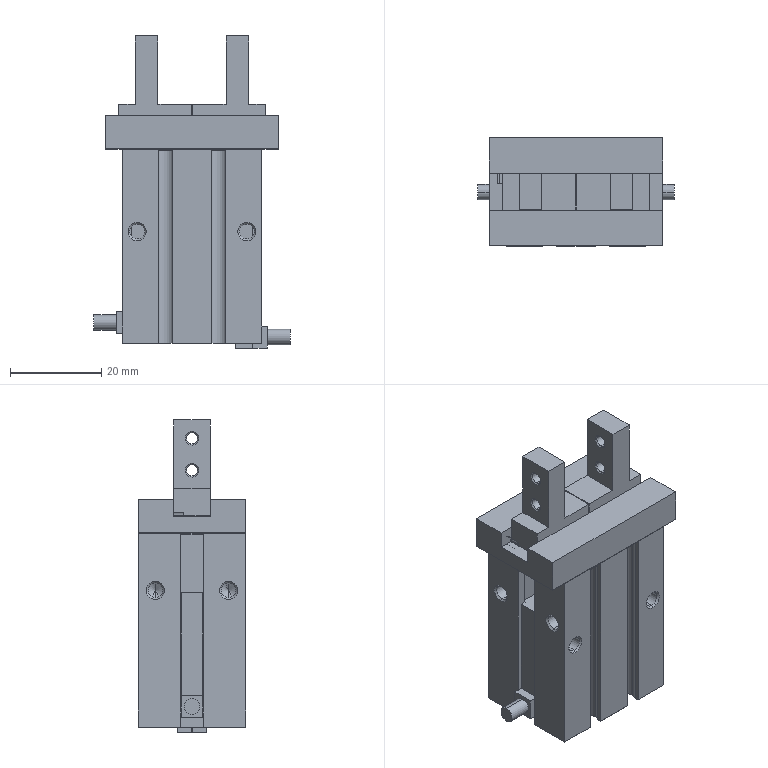Part | STEP file | Mount electronic clip cylinder MHZ2-16D-Y69A (14.9) | 1 solid | 458 faces | box 43.02 x 23.6 x 68.3 mm | volume 34069 mm3 | plane 272 | spline 94 | cylinder 48 | cone 44 | commonest cylinder face diameters 3.24 x16 4.02 x12 2.46 x8 3.4 x4 4.48 x4 3 x2